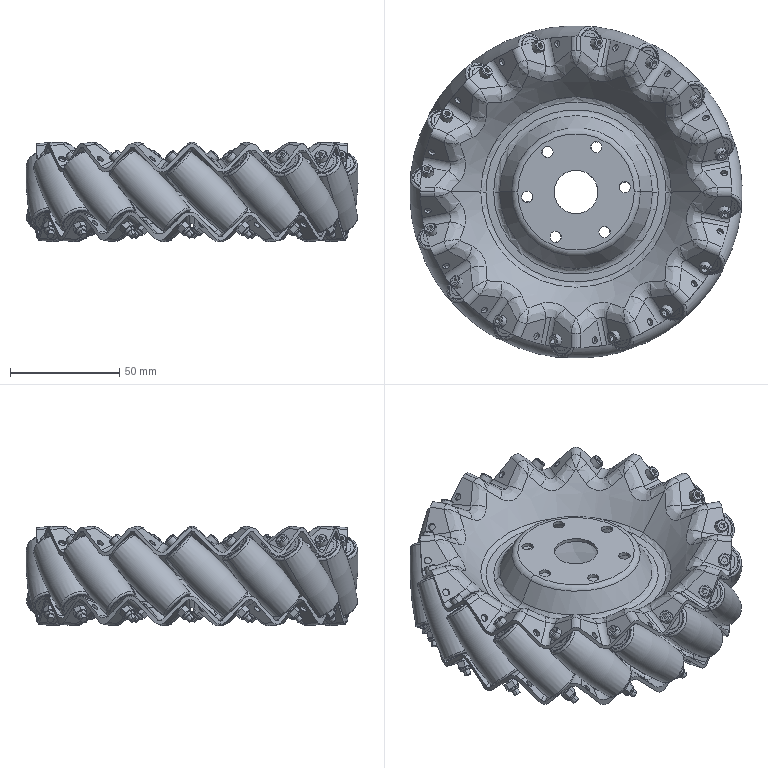Part | SolidWorks | features BaseBody 114, ICE 1 | 114 solids | 1934 faces | box 152.18 x 152.18 x 45.547 mm | volume 218308 mm3 | cylinder 796 | plane 632 | spline 286 | torus 140 | cone 80 | commonest cylinder face diameters 5 x128 10 x128 3.2 x108 3 x96 6.35 x78 13 x64